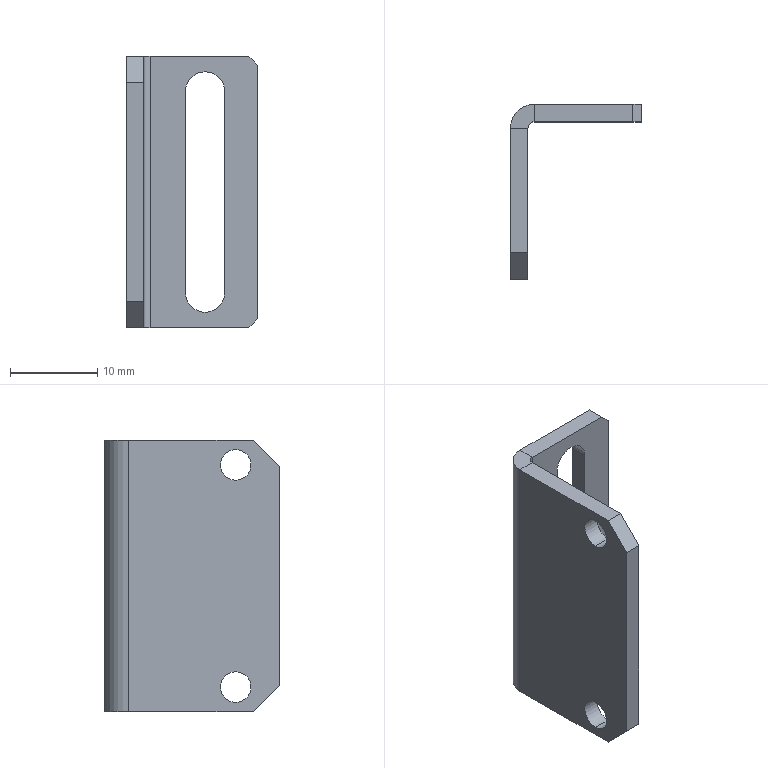Part | STEP file | 11-FG-SZ02311 | 1 solid | 27 faces | box 15 x 20 x 31 mm | volume 1702 mm3 | plane 18 | cylinder 9 | commonest cylinder face diameters 3.5 x4 4.5 x3 1.473 x1 5.473 x1
STEP:
#1=CARTESIAN_POINT('',(9.,18.,29.25));
#2=VERTEX_POINT('',#1);
#3=CARTESIAN_POINT('',(11.25,18.,27.));
#4=VERTEX_POINT('',#3);
#5=CARTESIAN_POINT('',(9.,18.,27.));
#6=DIRECTION('',(0.,1.,0.));
#7=DIRECTION('',(0.,0.,1.));
#8=AXIS2_PLACEMENT_3D('',#5,#6,#7);
#9=CIRCLE('',#8,2.25);
#10=EDGE_CURVE('',#2,#4,#9,.T.);
#11=ORIENTED_EDGE('',*,*,#10,.F.);
#12=CARTESIAN_POINT('',(9.,20.,29.25));
#13=VERTEX_POINT('',#12);
#14=CARTESIAN_POINT('',(9.,10.,29.25));
#15=DIRECTION('',(0.,1.,0.));
#16=VECTOR('',#15,1000.);
#17=LINE('',#14,#16);
#18=EDGE_CURVE('',#2,#13,#17,.T.);
#19=ORIENTED_EDGE('',*,*,#18,.T.);
#20=CARTESIAN_POINT('',(11.25,20.,27.));
#21=VERTEX_POINT('',#20);
#22=CARTESIAN_POINT('',(9.,20.,27.));
#23=DIRECTION('',(0.,1.,0.));
#24=DIRECTION('',(0.,0.,1.));
#25=AXIS2_PLACEMENT_3D('',#22,#23,#24);
#26=CIRCLE('',#25,2.25);
#27=EDGE_CURVE('',#13,#21,#26,.T.);
#28=ORIENTED_EDGE('',*,*,#27,.T.);
#29=CARTESIAN_POINT('',(11.25,10.,27.));
#30=DIRECTION('',(0.,1.,0.));
#31=VECTOR('',#30,1000.);
#32=LINE('',#29,#31);
#33=EDGE_CURVE('',#4,#21,#32,.T.);
#34=ORIENTED_EDGE('',*,*,#33,.F.);
#35=EDGE_LOOP('',(#11,#19,#28,#34));
#36=FACE_OUTER_BOUND('',#35,.T.);
#37=CARTESIAN_POINT('',(9.,10.,27.));
#38=DIRECTION('',(0.,1.,0.));
#39=DIRECTION('',(0.,0.,1.));
#40=AXIS2_PLACEMENT_3D('',#37,#38,#39);
#41=CYLINDRICAL_SURFACE('',#40,2.25);
#42=ADVANCED_FACE('',(#36),#41,.F.);
#43=CARTESIAN_POINT('',(2.,5.,26.45));
#44=VERTEX_POINT('',#43);
#45=CARTESIAN_POINT('',(2.,5.,29.95));
#46=VERTEX_POINT('',#45);
#47=CARTESIAN_POINT('',(2.,5.,28.2));
#48=DIRECTION('',(-1.,0.,0.));
#49=DIRECTION('',(0.,0.,1.));
#50=AXIS2_PLACEMENT_3D('',#47,#48,#49);
#51=CIRCLE('',#50,1.75);
#52=EDGE_CURVE('',#44,#46,#51,.T.);
#53=ORIENTED_EDGE('',*,*,#52,.F.);
#54=CARTESIAN_POINT('',(0.,5.,26.45));
#55=VERTEX_POINT('',#54);
#56=CARTESIAN_POINT('',(0.,5.,26.45));
#57=DIRECTION('',(-1.,0.,0.));
#58=VECTOR('',#57,1000.);
#59=LINE('',#56,#58);
#60=EDGE_CURVE('',#44,#55,#59,.T.);
#61=ORIENTED_EDGE('',*,*,#60,.T.);
#62=CARTESIAN_POINT('',(0.,5.,29.95));
#63=VERTEX_POINT('',#62);
#64=CARTESIAN_POINT('',(0.,5.,28.2));
#65=DIRECTION('',(-1.,0.,0.));
#66=DIRECTION('',(0.,0.,1.));
#67=AXIS2_PLACEMENT_3D('',#64,#65,#66);
#68=CIRCLE('',#67,1.75);
#69=EDGE_CURVE('',#55,#63,#68,.T.);
#70=ORIENTED_EDGE('',*,*,#69,.T.);
#71=CARTESIAN_POINT('',(0.,5.,29.95));
#72=DIRECTION('',(-1.,0.,0.));
#73=VECTOR('',#72,1000.);
#74=LINE('',#71,#73);
#75=EDGE_CURVE('',#46,#63,#74,.T.);
#76=ORIENTED_EDGE('',*,*,#75,.F.);
#77=EDGE_LOOP('',(#53,#61,#70,#76));
#78=FACE_OUTER_BOUND('',#77,.T.);
#79=CARTESIAN_POINT('',(0.,5.,28.2));
#80=DIRECTION('',(-1.,0.,0.));
#81=DIRECTION('',(0.,0.,1.));
#82=AXIS2_PLACEMENT_3D('',#79,#80,#81);
#83=CYLINDRICAL_SURFACE('',#82,1.75);
#84=ADVANCED_FACE('',(#78),#83,.F.);
#85=CARTESIAN_POINT('',(2.,5.,1.05));
#86=VERTEX_POINT('',#85);
#87=CARTESIAN_POINT('',(2.,5.,4.55));
#88=VERTEX_POINT('',#87);
#89=CARTESIAN_POINT('',(2.,5.,2.8));
#90=DIRECTION('',(-1.,0.,0.));
#91=DIRECTION('',(0.,0.,1.));
#92=AXIS2_PLACEMENT_3D('',#89,#90,#91);
#93=CIRCLE('',#92,1.75);
#94=EDGE_CURVE('',#86,#88,#93,.T.);
#95=ORIENTED_EDGE('',*,*,#94,.F.);
#96=CARTESIAN_POINT('',(0.,5.,1.05));
#97=VERTEX_POINT('',#96);
#98=CARTESIAN_POINT('',(0.,5.,1.05));
#99=DIRECTION('',(-1.,0.,0.));
#100=VECTOR('',#99,1000.);
#101=LINE('',#98,#100);
#102=EDGE_CURVE('',#86,#97,#101,.T.);
#103=ORIENTED_EDGE('',*,*,#102,.T.);
#104=CARTESIAN_POINT('',(0.,5.,4.55));
#105=VERTEX_POINT('',#104);
#106=CARTESIAN_POINT('',(0.,5.,2.8));
#107=DIRECTION('',(-1.,0.,0.));
#108=DIRECTION('',(0.,0.,1.));
#109=AXIS2_PLACEMENT_3D('',#106,#107,#108);
#110=CIRCLE('',#109,1.75);
#111=EDGE_CURVE('',#97,#105,#110,.T.);
#112=ORIENTED_EDGE('',*,*,#111,.T.);
#113=CARTESIAN_POINT('',(0.,5.,4.55));
#114=DIRECTION('',(-1.,0.,0.));
#115=VECTOR('',#114,1000.);
#116=LINE('',#113,#115);
#117=EDGE_CURVE('',#88,#105,#116,.T.);
#118=ORIENTED_EDGE('',*,*,#117,.F.);
#119=EDGE_LOOP('',(#95,#103,#112,#118));
#120=FACE_OUTER_BOUND('',#119,.T.);
#121=CARTESIAN_POINT('',(0.,5.,2.8));
#122=DIRECTION('',(-1.,0.,0.));
#123=DIRECTION('',(0.,0.,1.));
#124=AXIS2_PLACEMENT_3D('',#121,#122,#123);
#125=CYLINDRICAL_SURFACE('',#124,1.75);
#126=ADVANCED_FACE('',(#120),#125,.F.);
#127=CARTESIAN_POINT('',(2.737,20.,31.));
#128=VERTEX_POINT('',#127);
#129=CARTESIAN_POINT('',(2.737,18.,31.));
#130=VERTEX_POINT('',#129);
#131=CARTESIAN_POINT('',(2.737,20.,31.));
#132=DIRECTION('',(0.,-1.,0.));
#133=VECTOR('',#132,1000.);
#134=LINE('',#131,#133);
#135=EDGE_CURVE('',#128,#130,#134,.T.);
#136=ORIENTED_EDGE('',*,*,#135,.F.);
#137=CARTESIAN_POINT('',(0.,17.263,31.));
#138=VERTEX_POINT('',#137);
#139=CARTESIAN_POINT('',(2.737,17.263,31.));
#140=DIRECTION('',(0.,0.,-1.));
#141=DIRECTION('',(1.,0.,0.));
#142=AXIS2_PLACEMENT_3D('',#139,#140,#141);
#143=CIRCLE('',#142,2.737);
#144=EDGE_CURVE('',#138,#128,#143,.T.);
#145=ORIENTED_EDGE('',*,*,#144,.F.);
#146=CARTESIAN_POINT('',(2.,17.263,31.));
#147=VERTEX_POINT('',#146);
#148=CARTESIAN_POINT('',(2.,17.263,31.));
#149=DIRECTION('',(-1.,0.,0.));
#150=VECTOR('',#149,1000.);
#151=LINE('',#148,#150);
#152=EDGE_CURVE('',#147,#138,#151,.T.);
#153=ORIENTED_EDGE('',*,*,#152,.F.);
#154=CARTESIAN_POINT('',(2.737,17.263,31.));
#155=DIRECTION('',(0.,0.,-1.));
#156=DIRECTION('',(1.,0.,0.));
#157=AXIS2_PLACEMENT_3D('',#154,#155,#156);
#158=CIRCLE('',#157,0.7366);
#159=EDGE_CURVE('',#147,#130,#158,.T.);
#160=ORIENTED_EDGE('',*,*,#159,.T.);
#161=EDGE_LOOP('',(#136,#145,#153,#160));
#162=FACE_OUTER_BOUND('',#161,.T.);
#163=CARTESIAN_POINT('',(2.737,20.,31.));
#164=DIRECTION('',(0.,0.,1.));
#165=DIRECTION('',(1.,0.,0.));
#166=AXIS2_PLACEMENT_3D('',#163,#164,#165);
#167=PLANE('',#166);
#168=ADVANCED_FACE('',(#162),#167,.T.);
#169=CARTESIAN_POINT('',(14.,18.,31.));
#170=VERTEX_POINT('',#169);
#171=CARTESIAN_POINT('',(0.,18.,31.));
#172=DIRECTION('',(1.,0.,0.));
#173=VECTOR('',#172,1000.);
#174=LINE('',#171,#173);
#175=EDGE_CURVE('',#130,#170,#174,.T.);
#176=ORIENTED_EDGE('',*,*,#175,.T.);
#177=CARTESIAN_POINT('',(14.,20.,31.));
#178=VERTEX_POINT('',#177);
#179=CARTESIAN_POINT('',(14.,17.263,31.));
#180=DIRECTION('',(0.,1.,0.));
#181=VECTOR('',#180,1000.);
#182=LINE('',#179,#181);
#183=EDGE_CURVE('',#170,#178,#182,.T.);
#184=ORIENTED_EDGE('',*,*,#183,.T.);
#185=CARTESIAN_POINT('',(0.,20.,31.));
#186=DIRECTION('',(1.,0.,0.));
#187=VECTOR('',#186,1000.);
#188=LINE('',#185,#187);
#189=EDGE_CURVE('',#128,#178,#188,.T.);
#190=ORIENTED_EDGE('',*,*,#189,.F.);
#191=ORIENTED_EDGE('',*,*,#135,.T.);
#192=EDGE_LOOP('',(#176,#184,#190,#191));
#193=FACE_OUTER_BOUND('',#192,.T.);
#194=CARTESIAN_POINT('',(2.,17.263,31.));
#195=DIRECTION('',(0.,0.,1.));
#196=DIRECTION('',(1.,0.,0.));
#197=AXIS2_PLACEMENT_3D('',#194,#195,#196);
#198=PLANE('',#197);
#199=ADVANCED_FACE('',(#193),#198,.T.);
#200=CARTESIAN_POINT('',(0.,17.263,0.));
#201=VERTEX_POINT('',#200);
#202=CARTESIAN_POINT('',(2.,17.263,0.));
#203=VERTEX_POINT('',#202);
#204=CARTESIAN_POINT('',(0.,17.263,0.));
#205=DIRECTION('',(1.,0.,0.));
#206=VECTOR('',#205,1000.);
#207=LINE('',#204,#206);
#208=EDGE_CURVE('',#201,#203,#207,.T.);
#209=ORIENTED_EDGE('',*,*,#208,.F.);
#210=CARTESIAN_POINT('',(2.737,20.,0.));
#211=VERTEX_POINT('',#210);
#212=CARTESIAN_POINT('',(2.737,17.263,0.));
#213=DIRECTION('',(0.,0.,-1.));
#214=DIRECTION('',(1.,0.,0.));
#215=AXIS2_PLACEMENT_3D('',#212,#213,#214);
#216=CIRCLE('',#215,2.737);
#217=EDGE_CURVE('',#201,#211,#216,.T.);
#218=ORIENTED_EDGE('',*,*,#217,.T.);
#219=CARTESIAN_POINT('',(2.737,18.,0.));
#220=VERTEX_POINT('',#219);
#221=CARTESIAN_POINT('',(2.737,18.,0.));
#222=DIRECTION('',(0.,1.,0.));
#223=VECTOR('',#222,1000.);
#224=LINE('',#221,#223);
#225=EDGE_CURVE('',#220,#211,#224,.T.);
#226=ORIENTED_EDGE('',*,*,#225,.F.);
#227=CARTESIAN_POINT('',(2.737,17.263,0.));
#228=DIRECTION('',(0.,0.,-1.));
#229=DIRECTION('',(1.,0.,0.));
#230=AXIS2_PLACEMENT_3D('',#227,#228,#229);
#231=CIRCLE('',#230,0.7366);
#232=EDGE_CURVE('',#203,#220,#231,.T.);
#233=ORIENTED_EDGE('',*,*,#232,.F.);
#234=EDGE_LOOP('',(#209,#218,#226,#233));
#235=FACE_OUTER_BOUND('',#234,.T.);
#236=CARTESIAN_POINT('',(0.,17.263,0.));
#237=DIRECTION('',(0.,0.,-1.));
#238=DIRECTION('',(-1.,0.,0.));
#239=AXIS2_PLACEMENT_3D('',#236,#237,#238);
#240=PLANE('',#239);
#241=ADVANCED_FACE('',(#235),#240,.T.);
#242=CARTESIAN_POINT('',(2.,3.,0.));
#243=VERTEX_POINT('',#242);
#244=CARTESIAN_POINT('',(2.,0.,0.));
#245=DIRECTION('',(0.,1.,0.));
#246=VECTOR('',#245,1000.);
#247=LINE('',#244,#246);
#248=EDGE_CURVE('',#243,#203,#247,.T.);
#249=ORIENTED_EDGE('',*,*,#248,.F.);
#250=CARTESIAN_POINT('',(0.,3.,0.));
#251=VERTEX_POINT('',#250);
#252=CARTESIAN_POINT('',(2.737,3.,0.));
#253=DIRECTION('',(-1.,0.,0.));
#254=VECTOR('',#253,1000.);
#255=LINE('',#252,#254);
#256=EDGE_CURVE('',#243,#251,#255,.T.);
#257=ORIENTED_EDGE('',*,*,#256,.T.);
#258=CARTESIAN_POINT('',(0.,0.,0.));
#259=DIRECTION('',(0.,1.,0.));
#260=VECTOR('',#259,1000.);
#261=LINE('',#258,#260);
#262=EDGE_CURVE('',#251,#201,#261,.T.);
#263=ORIENTED_EDGE('',*,*,#262,.T.);
#264=ORIENTED_EDGE('',*,*,#208,.T.);
#265=EDGE_LOOP('',(#249,#257,#263,#264));
#266=FACE_OUTER_BOUND('',#265,.T.);
#267=CARTESIAN_POINT('',(2.737,18.,0.));
#268=DIRECTION('',(0.,0.,-1.));
#269=DIRECTION('',(-1.,0.,0.));
#270=AXIS2_PLACEMENT_3D('',#267,#268,#269);
#271=PLANE('',#270);
#272=ADVANCED_FACE('',(#266),#271,.T.);
#273=CARTESIAN_POINT('',(11.25,18.,4.));
#274=VERTEX_POINT('',#273);
#275=CARTESIAN_POINT('',(11.25,18.,31.));
#276=DIRECTION('',(0.,0.,-1.));
#277=VECTOR('',#276,1000.);
#278=LINE('',#275,#277);
#279=EDGE_CURVE('',#4,#274,#278,.T.);
#280=ORIENTED_EDGE('',*,*,#279,.T.);
#281=CARTESIAN_POINT('',(6.75,18.,4.));
#282=VERTEX_POINT('',#281);
#283=CARTESIAN_POINT('',(9.,18.,4.));
#284=DIRECTION('',(0.,1.,0.));
#285=DIRECTION('',(0.,0.,1.));
#286=AXIS2_PLACEMENT_3D('',#283,#284,#285);
#287=CIRCLE('',#286,2.25);
#288=EDGE_CURVE('',#274,#282,#287,.T.);
#289=ORIENTED_EDGE('',*,*,#288,.T.);
#290=CARTESIAN_POINT('',(6.75,18.,27.));
#291=VERTEX_POINT('',#290);
#292=CARTESIAN_POINT('',(6.75,18.,31.));
#293=DIRECTION('',(0.,0.,1.));
#294=VECTOR('',#293,1000.);
#295=LINE('',#292,#294);
#296=EDGE_CURVE('',#282,#291,#295,.T.);
#297=ORIENTED_EDGE('',*,*,#296,.T.);
#298=CARTESIAN_POINT('',(9.,18.,27.));
#299=DIRECTION('',(0.,1.,0.));
#300=DIRECTION('',(0.,0.,1.));
#301=AXIS2_PLACEMENT_3D('',#298,#299,#300);
#302=CIRCLE('',#301,2.25);
#303=EDGE_CURVE('',#291,#2,#302,.T.);
#304=ORIENTED_EDGE('',*,*,#303,.T.);
#305=ORIENTED_EDGE('',*,*,#10,.T.);
#306=EDGE_LOOP('',(#280,#289,#297,#304,#305));
#307=FACE_BOUND('',#306,.T.);
#308=CARTESIAN_POINT('',(14.,18.,0.));
#309=VERTEX_POINT('',#308);
#310=CARTESIAN_POINT('',(0.,18.,0.));
#311=DIRECTION('',(1.,0.,0.));
#312=VECTOR('',#311,1000.);
#313=LINE('',#310,#312);
#314=EDGE_CURVE('',#220,#309,#313,.T.);
#315=ORIENTED_EDGE('',*,*,#314,.T.);
#316=CARTESIAN_POINT('',(15.,18.,1.));
#317=VERTEX_POINT('',#316);
#318=CARTESIAN_POINT('',(14.,18.,0.));
#319=DIRECTION('',(0.7071,0.,0.7071));
#320=VECTOR('',#319,1000.);
#321=LINE('',#318,#320);
#322=EDGE_CURVE('',#309,#317,#321,.T.);
#323=ORIENTED_EDGE('',*,*,#322,.T.);
#324=CARTESIAN_POINT('',(15.,18.,30.));
#325=VERTEX_POINT('',#324);
#326=CARTESIAN_POINT('',(15.,18.,31.));
#327=DIRECTION('',(0.,0.,-1.));
#328=VECTOR('',#327,1000.);
#329=LINE('',#326,#328);
#330=EDGE_CURVE('',#325,#317,#329,.T.);
#331=ORIENTED_EDGE('',*,*,#330,.F.);
#332=CARTESIAN_POINT('',(15.,18.,30.));
#333=DIRECTION('',(-0.7071,0.,0.7071));
#334=VECTOR('',#333,1000.);
#335=LINE('',#332,#334);
#336=EDGE_CURVE('',#325,#170,#335,.T.);
#337=ORIENTED_EDGE('',*,*,#336,.T.);
#338=ORIENTED_EDGE('',*,*,#175,.F.);
#339=CARTESIAN_POINT('',(2.737,18.,31.));
#340=DIRECTION('',(0.,0.,-1.));
#341=VECTOR('',#340,1000.);
#342=LINE('',#339,#341);
#343=EDGE_CURVE('',#130,#220,#342,.T.);
#344=ORIENTED_EDGE('',*,*,#343,.T.);
#345=EDGE_LOOP('',(#315,#323,#331,#337,#338,#344));
#346=FACE_OUTER_BOUND('',#345,.T.);
#347=CARTESIAN_POINT('',(0.,18.,31.));
#348=DIRECTION('',(0.,1.,0.));
#349=DIRECTION('',(0.,0.,1.));
#350=AXIS2_PLACEMENT_3D('',#347,#348,#349);
#351=PLANE('',#350);
#352=ADVANCED_FACE('',(#307,#346),#351,.F.);
#353=ORIENTED_EDGE('',*,*,#330,.T.);
#354=CARTESIAN_POINT('',(15.,20.,1.));
#355=VERTEX_POINT('',#354);
#356=CARTESIAN_POINT('',(15.,20.,1.));
#357=DIRECTION('',(0.,1.,0.));
#358=VECTOR('',#357,1000.);
#359=LINE('',#356,#358);
#360=EDGE_CURVE('',#317,#355,#359,.T.);
#361=ORIENTED_EDGE('',*,*,#360,.T.);
#362=CARTESIAN_POINT('',(15.,20.,30.));
#363=VERTEX_POINT('',#362);
#364=CARTESIAN_POINT('',(15.,20.,31.));
#365=DIRECTION('',(0.,0.,-1.));
#366=VECTOR('',#365,1000.);
#367=LINE('',#364,#366);
#368=EDGE_CURVE('',#363,#355,#367,.T.);
#369=ORIENTED_EDGE('',*,*,#368,.F.);
#370=CARTESIAN_POINT('',(15.,20.,30.));
#371=DIRECTION('',(0.,-1.,0.));
#372=VECTOR('',#371,1000.);
#373=LINE('',#370,#372);
#374=EDGE_CURVE('',#363,#325,#373,.T.);
#375=ORIENTED_EDGE('',*,*,#374,.T.);
#376=EDGE_LOOP('',(#353,#361,#369,#375));
#377=FACE_OUTER_BOUND('',#376,.T.);
#378=CARTESIAN_POINT('',(15.,20.,31.));
#379=DIRECTION('',(1.,0.,0.));
#380=DIRECTION('',(0.,0.,-1.));
#381=AXIS2_PLACEMENT_3D('',#378,#379,#380);
#382=PLANE('',#381);
#383=ADVANCED_FACE('',(#377),#382,.T.);
#384=CARTESIAN_POINT('',(11.25,20.,4.));
#385=VERTEX_POINT('',#384);
#386=CARTESIAN_POINT('',(6.75,20.,4.));
#387=VERTEX_POINT('',#386);
#388=CARTESIAN_POINT('',(9.,20.,4.));
#389=DIRECTION('',(0.,1.,0.));
#390=DIRECTION('',(0.,0.,1.));
#391=AXIS2_PLACEMENT_3D('',#388,#389,#390);
#392=CIRCLE('',#391,2.25);
#393=EDGE_CURVE('',#385,#387,#392,.T.);
#394=ORIENTED_EDGE('',*,*,#393,.F.);
#395=CARTESIAN_POINT('',(11.25,20.,4.));
#396=DIRECTION('',(0.,0.,-1.));
#397=VECTOR('',#396,1000.);
#398=LINE('',#395,#397);
#399=EDGE_CURVE('',#21,#385,#398,.T.);
#400=ORIENTED_EDGE('',*,*,#399,.F.);
#401=ORIENTED_EDGE('',*,*,#27,.F.);
#402=CARTESIAN_POINT('',(6.75,20.,27.));
#403=VERTEX_POINT('',#402);
#404=CARTESIAN_POINT('',(9.,20.,27.));
#405=DIRECTION('',(0.,1.,0.));
#406=DIRECTION('',(0.,0.,1.));
#407=AXIS2_PLACEMENT_3D('',#404,#405,#406);
#408=CIRCLE('',#407,2.25);
#409=EDGE_CURVE('',#403,#13,#408,.T.);
#410=ORIENTED_EDGE('',*,*,#409,.F.);
#411=CARTESIAN_POINT('',(6.75,20.,4.));
#412=DIRECTION('',(0.,0.,1.));
#413=VECTOR('',#412,1000.);
#414=LINE('',#411,#413);
#415=EDGE_CURVE('',#387,#403,#414,.T.);
#416=ORIENTED_EDGE('',*,*,#415,.F.);
#417=EDGE_LOOP('',(#394,#400,#401,#410,#416));
#418=FACE_BOUND('',#417,.T.);
#419=ORIENTED_EDGE('',*,*,#368,.T.);
#420=CARTESIAN_POINT('',(14.,20.,0.));
#421=VERTEX_POINT('',#420);
#422=CARTESIAN_POINT('',(22.5,20.,8.5));
#423=DIRECTION('',(-0.7071,0.,-0.7071));
#424=VECTOR('',#423,1000.);
#425=LINE('',#422,#424);
#426=EDGE_CURVE('',#355,#421,#425,.T.);
#427=ORIENTED_EDGE('',*,*,#426,.T.);
#428=CARTESIAN_POINT('',(0.,20.,0.));
#429=DIRECTION('',(1.,0.,0.));
#430=VECTOR('',#429,1000.);
#431=LINE('',#428,#430);
#432=EDGE_CURVE('',#211,#421,#431,.T.);
#433=ORIENTED_EDGE('',*,*,#432,.F.);
#434=CARTESIAN_POINT('',(2.737,20.,31.));
#435=DIRECTION('',(0.,0.,-1.));
#436=VECTOR('',#435,1000.);
#437=LINE('',#434,#436);
#438=EDGE_CURVE('',#128,#211,#437,.T.);
#439=ORIENTED_EDGE('',*,*,#438,.F.);
#440=ORIENTED_EDGE('',*,*,#189,.T.);
#441=CARTESIAN_POINT('',(7.,20.,38.));
#442=DIRECTION('',(0.7071,0.,-0.7071));
#443=VECTOR('',#442,1000.);
#444=LINE('',#441,#443);
#445=EDGE_CURVE('',#178,#363,#444,.T.);
#446=ORIENTED_EDGE('',*,*,#445,.T.);
#447=EDGE_LOOP('',(#419,#427,#433,#439,#440,#446));
#448=FACE_OUTER_BOUND('',#447,.T.);
#449=CARTESIAN_POINT('',(0.,20.,31.));
#450=DIRECTION('',(0.,1.,0.));
#451=DIRECTION('',(0.,0.,1.));
#452=AXIS2_PLACEMENT_3D('',#449,#450,#451);
#453=PLANE('',#452);
#454=ADVANCED_FACE('',(#418,#448),#453,.T.);
#455=ORIENTED_EDGE('',*,*,#217,.F.);
#456=CARTESIAN_POINT('',(0.,17.263,31.));
#457=DIRECTION('',(0.,0.,-1.));
#458=VECTOR('',#457,1000.);
#459=LINE('',#456,#458);
#460=EDGE_CURVE('',#138,#201,#459,.T.);
#461=ORIENTED_EDGE('',*,*,#460,.F.);
#462=ORIENTED_EDGE('',*,*,#144,.T.);
#463=ORIENTED_EDGE('',*,*,#438,.T.);
#464=EDGE_LOOP('',(#455,#461,#462,#463));
#465=FACE_OUTER_BOUND('',#464,.T.);
#466=CARTESIAN_POINT('',(2.737,17.263,31.));
#467=DIRECTION('',(0.,0.,-1.));
#468=DIRECTION('',(-1.,0.,0.));
#469=AXIS2_PLACEMENT_3D('',#466,#467,#468);
#470=CYLINDRICAL_SURFACE('',#469,2.737);
#471=ADVANCED_FACE('',(#465),#470,.T.);
#472=CARTESIAN_POINT('',(0.,5.,28.2));
#473=DIRECTION('',(-1.,0.,0.));
#474=DIRECTION('',(0.,0.,1.));
#475=AXIS2_PLACEMENT_3D('',#472,#473,#474);
#476=CIRCLE('',#475,1.75);
#477=EDGE_CURVE('',#63,#55,#476,.T.);
#478=ORIENTED_EDGE('',*,*,#477,.F.);
#479=ORIENTED_EDGE('',*,*,#69,.F.);
#480=EDGE_LOOP('',(#478,#479));
#481=FACE_BOUND('',#480,.T.);
#482=CARTESIAN_POINT('',(0.,5.,2.8));
#483=DIRECTION('',(-1.,0.,0.));
#484=DIRECTION('',(0.,0.,1.));
#485=AXIS2_PLACEMENT_3D('',#482,#483,#484);
#486=CIRCLE('',#485,1.75);
#487=EDGE_CURVE('',#105,#97,#486,.T.);
#488=ORIENTED_EDGE('',*,*,#487,.F.);
#489=ORIENTED_EDGE('',*,*,#111,.F.);
#490=EDGE_LOOP('',(#488,#489));
#491=FACE_BOUND('',#490,.T.);
#492=CARTESIAN_POINT('',(0.,0.,28.));
#493=VERTEX_POINT('',#492);
#494=CARTESIAN_POINT('',(0.,0.,3.));
#495=VERTEX_POINT('',#494);
#496=CARTESIAN_POINT('',(0.,0.,31.));
#497=DIRECTION('',(0.,0.,-1.));
#498=VECTOR('',#497,1000.);
#499=LINE('',#496,#498);
#500=EDGE_CURVE('',#493,#495,#499,.T.);
#501=ORIENTED_EDGE('',*,*,#500,.F.);
#502=CARTESIAN_POINT('',(0.,3.,31.));
#503=VERTEX_POINT('',#502);
#504=CARTESIAN_POINT('',(0.,1.5,29.5));
#505=DIRECTION('',(0.,0.7071,0.7071));
#506=VECTOR('',#505,1000.);
#507=LINE('',#504,#506);
#508=EDGE_CURVE('',#493,#503,#507,.T.);
#509=ORIENTED_EDGE('',*,*,#508,.T.);
#510=CARTESIAN_POINT('',(0.,0.,31.));
#511=DIRECTION('',(0.,1.,0.));
#512=VECTOR('',#511,1000.);
#513=LINE('',#510,#512);
#514=EDGE_CURVE('',#503,#138,#513,.T.);
#515=ORIENTED_EDGE('',*,*,#514,.T.);
#516=ORIENTED_EDGE('',*,*,#460,.T.);
#517=ORIENTED_EDGE('',*,*,#262,.F.);
#518=CARTESIAN_POINT('',(0.,-14.,17.));
#519=DIRECTION('',(0.,-0.7071,0.7071));
#520=VECTOR('',#519,1000.);
#521=LINE('',#518,#520);
#522=EDGE_CURVE('',#251,#495,#521,.T.);
#523=ORIENTED_EDGE('',*,*,#522,.T.);
#524=EDGE_LOOP('',(#501,#509,#515,#516,#517,#523));
#525=FACE_OUTER_BOUND('',#524,.T.);
#526=CARTESIAN_POINT('',(0.,0.,31.));
#527=DIRECTION('',(-1.,0.,0.));
#528=DIRECTION('',(0.,0.,1.));
#529=AXIS2_PLACEMENT_3D('',#526,#527,#528);
#530=PLANE('',#529);
#531=ADVANCED_FACE('',(#481,#491,#525),#530,.T.);
#532=CARTESIAN_POINT('',(2.,0.,28.));
#533=VERTEX_POINT('',#532);
#534=CARTESIAN_POINT('',(2.,0.,3.));
#535=VERTEX_POINT('',#534);
#536=CARTESIAN_POINT('',(2.,0.,31.));
#537=DIRECTION('',(0.,0.,-1.));
#538=VECTOR('',#537,1000.);
#539=LINE('',#536,#538);
#540=EDGE_CURVE('',#533,#535,#539,.T.);
#541=ORIENTED_EDGE('',*,*,#540,.F.);
#542=CARTESIAN_POINT('',(2.,0.,28.));
#543=DIRECTION('',(-1.,0.,0.));
#544=VECTOR('',#543,1000.);
#545=LINE('',#542,#544);
#546=EDGE_CURVE('',#533,#493,#545,.T.);
#547=ORIENTED_EDGE('',*,*,#546,.T.);
#548=ORIENTED_EDGE('',*,*,#500,.T.);
#549=CARTESIAN_POINT('',(2.,0.,3.));
#550=DIRECTION('',(1.,0.,0.));
#551=VECTOR('',#550,1000.);
#552=LINE('',#549,#551);
#553=EDGE_CURVE('',#495,#535,#552,.T.);
#554=ORIENTED_EDGE('',*,*,#553,.T.);
#555=EDGE_LOOP('',(#541,#547,#548,#554));
#556=FACE_OUTER_BOUND('',#555,.T.);
#557=CARTESIAN_POINT('',(2.,0.,31.));
#558=DIRECTION('',(0.,-1.,0.));
#559=DIRECTION('',(0.,0.,-1.));
#560=AXIS2_PLACEMENT_3D('',#557,#558,#559);
#561=PLANE('',#560);
#562=ADVANCED_FACE('',(#556),#561,.T.);
#563=CARTESIAN_POINT('',(2.,5.,28.2));
#564=DIRECTION('',(-1.,0.,0.));
#565=DIRECTION('',(0.,0.,1.));
#566=AXIS2_PLACEMENT_3D('',#563,#564,#565);
#567=CIRCLE('',#566,1.75);
#568=EDGE_CURVE('',#46,#44,#567,.T.);
#569=ORIENTED_EDGE('',*,*,#568,.T.);
#570=ORIENTED_EDGE('',*,*,#52,.T.);
#571=EDGE_LOOP('',(#569,#570));
#572=FACE_BOUND('',#571,.T.);
#573=CARTESIAN_POINT('',(2.,5.,2.8));
#574=DIRECTION('',(-1.,0.,0.));
#575=DIRECTION('',(0.,0.,1.));
#576=AXIS2_PLACEMENT_3D('',#573,#574,#575);
#577=CIRCLE('',#576,1.75);
#578=EDGE_CURVE('',#88,#86,#577,.T.);
#579=ORIENTED_EDGE('',*,*,#578,.T.);
#580=ORIENTED_EDGE('',*,*,#94,.T.);
#581=EDGE_LOOP('',(#579,#580));
#582=FACE_BOUND('',#581,.T.);
#583=CARTESIAN_POINT('',(2.,3.,31.));
#584=VERTEX_POINT('',#583);
#585=CARTESIAN_POINT('',(2.,0.,31.));
#586=DIRECTION('',(0.,1.,0.));
#587=VECTOR('',#586,1000.);
#588=LINE('',#585,#587);
#589=EDGE_CURVE('',#584,#147,#588,.T.);
#590=ORIENTED_EDGE('',*,*,#589,.F.);
#591=CARTESIAN_POINT('',(2.,0.,28.));
#592=DIRECTION('',(0.,-0.7071,-0.7071));
#593=VECTOR('',#592,1000.);
#594=LINE('',#591,#593);
#595=EDGE_CURVE('',#584,#533,#594,.T.);
#596=ORIENTED_EDGE('',*,*,#595,.T.);
#597=ORIENTED_EDGE('',*,*,#540,.T.);
#598=CARTESIAN_POINT('',(2.,3.,0.));
#599=DIRECTION('',(0.,0.7071,-0.7071));
#600=VECTOR('',#599,1000.);
#601=LINE('',#598,#600);
#602=EDGE_CURVE('',#535,#243,#601,.T.);
#603=ORIENTED_EDGE('',*,*,#602,.T.);
#604=ORIENTED_EDGE('',*,*,#248,.T.);
#605=CARTESIAN_POINT('',(2.,17.263,31.));
#606=DIRECTION('',(0.,0.,-1.));
#607=VECTOR('',#606,1000.);
#608=LINE('',#605,#607);
#609=EDGE_CURVE('',#147,#203,#608,.T.);
#610=ORIENTED_EDGE('',*,*,#609,.F.);
#611=EDGE_LOOP('',(#590,#596,#597,#603,#604,#610));
#612=FACE_OUTER_BOUND('',#611,.T.);
#613=CARTESIAN_POINT('',(2.,0.,31.));
#614=DIRECTION('',(-1.,0.,0.));
#615=DIRECTION('',(0.,0.,1.));
#616=AXIS2_PLACEMENT_3D('',#613,#614,#615);
#617=PLANE('',#616);
#618=ADVANCED_FACE('',(#572,#582,#612),#617,.F.);
#619=ORIENTED_EDGE('',*,*,#232,.T.);
#620=ORIENTED_EDGE('',*,*,#343,.F.);
#621=ORIENTED_EDGE('',*,*,#159,.F.);
#622=ORIENTED_EDGE('',*,*,#609,.T.);
#623=EDGE_LOOP('',(#619,#620,#621,#622));
#624=FACE_OUTER_BOUND('',#623,.T.);
#625=CARTESIAN_POINT('',(2.737,17.263,31.));
#626=DIRECTION('',(0.,0.,-1.));
#627=DIRECTION('',(-1.,0.,0.));
#628=AXIS2_PLACEMENT_3D('',#625,#626,#627);
#629=CYLINDRICAL_SURFACE('',#628,0.7366);
#630=ADVANCED_FACE('',(#624),#629,.F.);
#631=ORIENTED_EDGE('',*,*,#514,.F.);
#632=CARTESIAN_POINT('',(2.737,3.,31.));
#633=DIRECTION('',(1.,0.,0.));
#634=VECTOR('',#633,1000.);
#635=LINE('',#632,#634);
#636=EDGE_CURVE('',#503,#584,#635,.T.);
#637=ORIENTED_EDGE('',*,*,#636,.T.);
#638=ORIENTED_EDGE('',*,*,#589,.T.);
#639=ORIENTED_EDGE('',*,*,#152,.T.);
#640=EDGE_LOOP('',(#631,#637,#638,#639));
#641=FACE_OUTER_BOUND('',#640,.T.);
#642=CARTESIAN_POINT('',(2.737,17.263,31.));
#643=DIRECTION('',(0.,0.,1.));
#644=DIRECTION('',(1.,0.,0.));
#645=AXIS2_PLACEMENT_3D('',#642,#643,#644);
#646=PLANE('',#645);
#647=ADVANCED_FACE('',(#641),#646,.T.);
#648=ORIENTED_EDGE('',*,*,#432,.T.);
#649=CARTESIAN_POINT('',(14.,18.,0.));
#650=DIRECTION('',(0.,-1.,0.));
#651=VECTOR('',#650,1000.);
#652=LINE('',#649,#651);
#653=EDGE_CURVE('',#421,#309,#652,.T.);
#654=ORIENTED_EDGE('',*,*,#653,.T.);
#655=ORIENTED_EDGE('',*,*,#314,.F.);
#656=ORIENTED_EDGE('',*,*,#225,.T.);
#657=EDGE_LOOP('',(#648,#654,#655,#656));
#658=FACE_OUTER_BOUND('',#657,.T.);
#659=CARTESIAN_POINT('',(2.737,17.263,0.));
#660=DIRECTION('',(0.,0.,1.));
#661=DIRECTION('',(1.,0.,0.));
#662=AXIS2_PLACEMENT_3D('',#659,#660,#661);
#663=PLANE('',#662);
#664=ADVANCED_FACE('',(#658),#663,.F.);
#665=ORIENTED_EDGE('',*,*,#102,.F.);
#666=ORIENTED_EDGE('',*,*,#578,.F.);
#667=ORIENTED_EDGE('',*,*,#117,.T.);
#668=ORIENTED_EDGE('',*,*,#487,.T.);
#669=EDGE_LOOP('',(#665,#666,#667,#668));
#670=FACE_OUTER_BOUND('',#669,.T.);
#671=CARTESIAN_POINT('',(0.,5.,2.8));
#672=DIRECTION('',(-1.,0.,0.));
#673=DIRECTION('',(0.,0.,1.));
#674=AXIS2_PLACEMENT_3D('',#671,#672,#673);
#675=CYLINDRICAL_SURFACE('',#674,1.75);
#676=ADVANCED_FACE('',(#670),#675,.F.);
#677=ORIENTED_EDGE('',*,*,#60,.F.);
#678=ORIENTED_EDGE('',*,*,#568,.F.);
#679=ORIENTED_EDGE('',*,*,#75,.T.);
#680=ORIENTED_EDGE('',*,*,#477,.T.);
#681=EDGE_LOOP('',(#677,#678,#679,#680));
#682=FACE_OUTER_BOUND('',#681,.T.);
#683=CARTESIAN_POINT('',(0.,5.,28.2));
#684=DIRECTION('',(-1.,0.,0.));
#685=DIRECTION('',(0.,0.,1.));
#686=AXIS2_PLACEMENT_3D('',#683,#684,#685);
#687=CYLINDRICAL_SURFACE('',#686,1.75);
#688=ADVANCED_FACE('',(#682),#687,.F.);
#689=ORIENTED_EDGE('',*,*,#595,.F.);
#690=ORIENTED_EDGE('',*,*,#636,.F.);
#691=ORIENTED_EDGE('',*,*,#508,.F.);
#692=ORIENTED_EDGE('',*,*,#546,.F.);
#693=EDGE_LOOP('',(#689,#690,#691,#692));
#694=FACE_OUTER_BOUND('',#693,.T.);
#695=CARTESIAN_POINT('',(2.,0.,28.));
#696=DIRECTION('',(0.,0.7071,-0.7071));
#697=DIRECTION('',(-1.,0.,0.));
#698=AXIS2_PLACEMENT_3D('',#695,#696,#697);
#699=PLANE('',#698);
#700=ADVANCED_FACE('',(#694),#699,.F.);
#701=ORIENTED_EDGE('',*,*,#602,.F.);
#702=ORIENTED_EDGE('',*,*,#553,.F.);
#703=ORIENTED_EDGE('',*,*,#522,.F.);
#704=ORIENTED_EDGE('',*,*,#256,.F.);
#705=EDGE_LOOP('',(#701,#702,#703,#704));
#706=FACE_OUTER_BOUND('',#705,.T.);
#707=CARTESIAN_POINT('',(2.737,3.,0.));
#708=DIRECTION('',(0.,0.7071,0.7071));
#709=DIRECTION('',(-1.,0.,0.));
#710=AXIS2_PLACEMENT_3D('',#707,#708,#709);
#711=PLANE('',#710);
#712=ADVANCED_FACE('',(#706),#711,.F.);
#713=CARTESIAN_POINT('',(11.25,10.,4.));
#714=DIRECTION('',(0.,1.,0.));
#715=VECTOR('',#714,1000.);
#716=LINE('',#713,#715);
#717=EDGE_CURVE('',#274,#385,#716,.T.);
#718=ORIENTED_EDGE('',*,*,#717,.T.);
#719=ORIENTED_EDGE('',*,*,#393,.T.);
#720=CARTESIAN_POINT('',(6.75,10.,4.));
#721=DIRECTION('',(0.,1.,0.));
#722=VECTOR('',#721,1000.);
#723=LINE('',#720,#722);
#724=EDGE_CURVE('',#282,#387,#723,.T.);
#725=ORIENTED_EDGE('',*,*,#724,.F.);
#726=ORIENTED_EDGE('',*,*,#288,.F.);
#727=EDGE_LOOP('',(#718,#719,#725,#726));
#728=FACE_OUTER_BOUND('',#727,.T.);
#729=CARTESIAN_POINT('',(9.,10.,4.));
#730=DIRECTION('',(0.,1.,0.));
#731=DIRECTION('',(0.,0.,1.));
#732=AXIS2_PLACEMENT_3D('',#729,#730,#731);
#733=CYLINDRICAL_SURFACE('',#732,2.25);
#734=ADVANCED_FACE('',(#728),#733,.F.);
#735=ORIENTED_EDGE('',*,*,#33,.T.);
#736=ORIENTED_EDGE('',*,*,#399,.T.);
#737=ORIENTED_EDGE('',*,*,#717,.F.);
#738=ORIENTED_EDGE('',*,*,#279,.F.);
#739=EDGE_LOOP('',(#735,#736,#737,#738));
#740=FACE_OUTER_BOUND('',#739,.T.);
#741=CARTESIAN_POINT('',(11.25,10.,4.));
#742=DIRECTION('',(1.,0.,0.));
#743=DIRECTION('',(0.,0.,-1.));
#744=AXIS2_PLACEMENT_3D('',#741,#742,#743);
#745=PLANE('',#744);
#746=ADVANCED_FACE('',(#740),#745,.F.);
#747=ORIENTED_EDGE('',*,*,#18,.F.);
#748=ORIENTED_EDGE('',*,*,#303,.F.);
#749=CARTESIAN_POINT('',(6.75,10.,27.));
#750=DIRECTION('',(0.,1.,0.));
#751=VECTOR('',#750,1000.);
#752=LINE('',#749,#751);
#753=EDGE_CURVE('',#291,#403,#752,.T.);
#754=ORIENTED_EDGE('',*,*,#753,.T.);
#755=ORIENTED_EDGE('',*,*,#409,.T.);
#756=EDGE_LOOP('',(#747,#748,#754,#755));
#757=FACE_OUTER_BOUND('',#756,.T.);
#758=CARTESIAN_POINT('',(9.,10.,27.));
#759=DIRECTION('',(0.,1.,0.));
#760=DIRECTION('',(0.,0.,1.));
#761=AXIS2_PLACEMENT_3D('',#758,#759,#760);
#762=CYLINDRICAL_SURFACE('',#761,2.25);
#763=ADVANCED_FACE('',(#757),#762,.F.);
#764=ORIENTED_EDGE('',*,*,#724,.T.);
#765=ORIENTED_EDGE('',*,*,#415,.T.);
#766=ORIENTED_EDGE('',*,*,#753,.F.);
#767=ORIENTED_EDGE('',*,*,#296,.F.);
#768=EDGE_LOOP('',(#764,#765,#766,#767));
#769=FACE_OUTER_BOUND('',#768,.T.);
#770=CARTESIAN_POINT('',(6.75,10.,4.));
#771=DIRECTION('',(-1.,0.,0.));
#772=DIRECTION('',(0.,0.,1.));
#773=AXIS2_PLACEMENT_3D('',#770,#771,#772);
#774=PLANE('',#773);
#775=ADVANCED_FACE('',(#769),#774,.F.);
#776=ORIENTED_EDGE('',*,*,#426,.F.);
#777=ORIENTED_EDGE('',*,*,#360,.F.);
#778=ORIENTED_EDGE('',*,*,#322,.F.);
#779=ORIENTED_EDGE('',*,*,#653,.F.);
#780=EDGE_LOOP('',(#776,#777,#778,#779));
#781=FACE_OUTER_BOUND('',#780,.T.);
#782=CARTESIAN_POINT('',(14.,17.263,0.));
#783=DIRECTION('',(0.7071,0.,-0.7071));
#784=DIRECTION('',(0.,1.,0.));
#785=AXIS2_PLACEMENT_3D('',#782,#783,#784);
#786=PLANE('',#785);
#787=ADVANCED_FACE('',(#781),#786,.T.);
#788=ORIENTED_EDGE('',*,*,#445,.F.);
#789=ORIENTED_EDGE('',*,*,#183,.F.);
#790=ORIENTED_EDGE('',*,*,#336,.F.);
#791=ORIENTED_EDGE('',*,*,#374,.F.);
#792=EDGE_LOOP('',(#788,#789,#790,#791));
#793=FACE_OUTER_BOUND('',#792,.T.);
#794=CARTESIAN_POINT('',(15.,20.,30.));
#795=DIRECTION('',(-0.7071,0.,-0.7071));
#796=DIRECTION('',(0.,-1.,0.));
#797=AXIS2_PLACEMENT_3D('',#794,#795,#796);
#798=PLANE('',#797);
#799=ADVANCED_FACE('',(#793),#798,.F.);
#800=CLOSED_SHELL('',(#42,#84,#126,#168,#199,#241,#272,#352,#383,#454,#471,#531,#562,#618,#630,#647,#664,#676,#688,#700,#712,#734,#746,#763,#775,#787,#799));
#801=MANIFOLD_SOLID_BREP('',#800);
#802=CARTESIAN_POINT('',(0.,0.,0.));
#803=DIRECTION('',(0.,0.,1.));
#804=DIRECTION('',(1.,0.,0.));
#805=AXIS2_PLACEMENT_3D('',#802,#803,#804);
#806=(LENGTH_UNIT()NAMED_UNIT(*)SI_UNIT(.MILLI.,.METRE.));
#807=UNCERTAINTY_MEASURE_WITH_UNIT(LENGTH_MEASURE(0.00001),#806,'','');
#808=(NAMED_UNIT(*)PLANE_ANGLE_UNIT()SI_UNIT($,.RADIAN.));
#809=(NAMED_UNIT(*)SI_UNIT($,.STERADIAN.)SOLID_ANGLE_UNIT());
#810=(GEOMETRIC_REPRESENTATION_CONTEXT(3)GLOBAL_UNCERTAINTY_ASSIGNED_CONTEXT((#807))GLOBAL_UNIT_ASSIGNED_CONTEXT((#806,#808,#809))REPRESENTATION_CONTEXT('',''));
#811=ADVANCED_BREP_SHAPE_REPRESENTATION('',(#801,#805),#810);